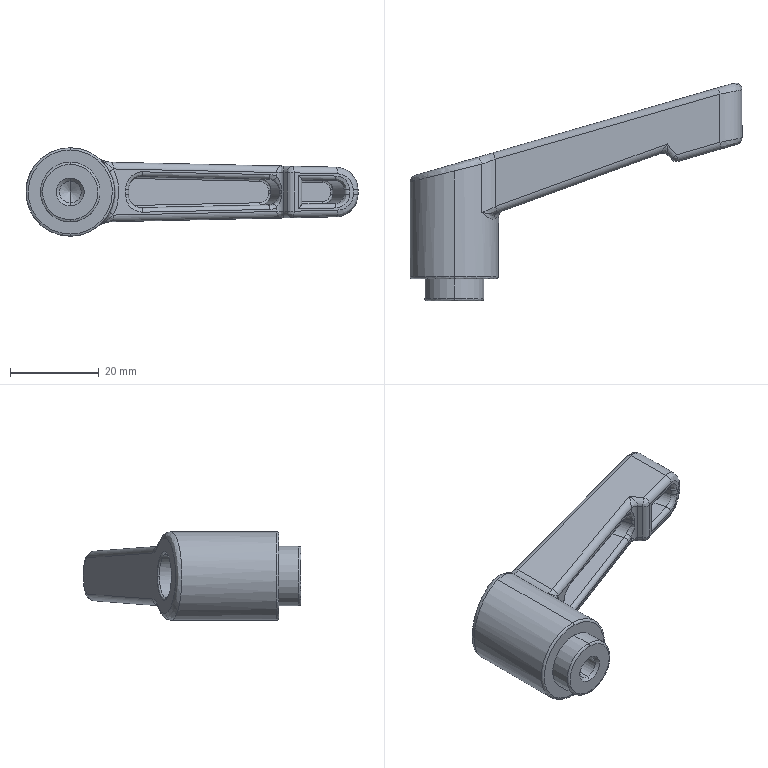Part | SolidWorks | 1 solid | 112 faces | box 75 x 49.204 x 20.002 mm | volume 13893 mm3 | cylinder 46 | spline 42 | plane 20 | cone 4 | commonest cylinder face diameters 3 x12 2 x10 1 x8 10 x4 4.917 x2 5 x2